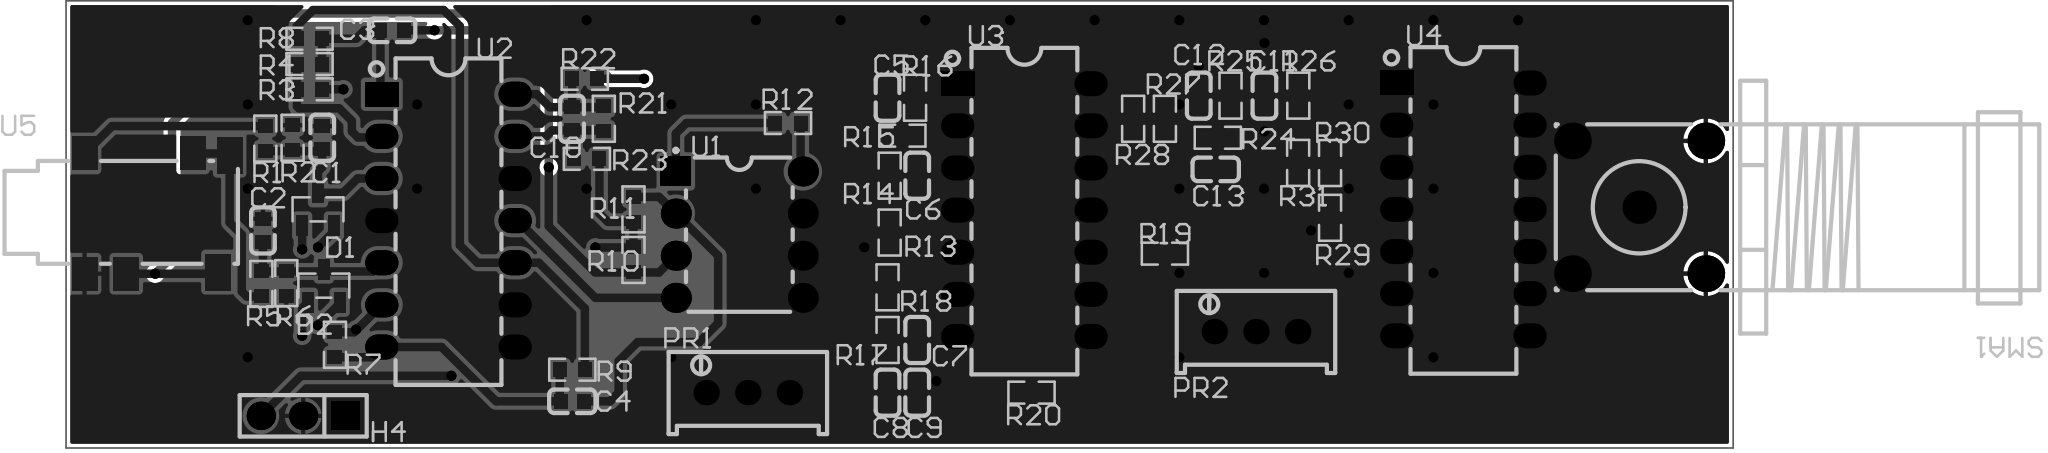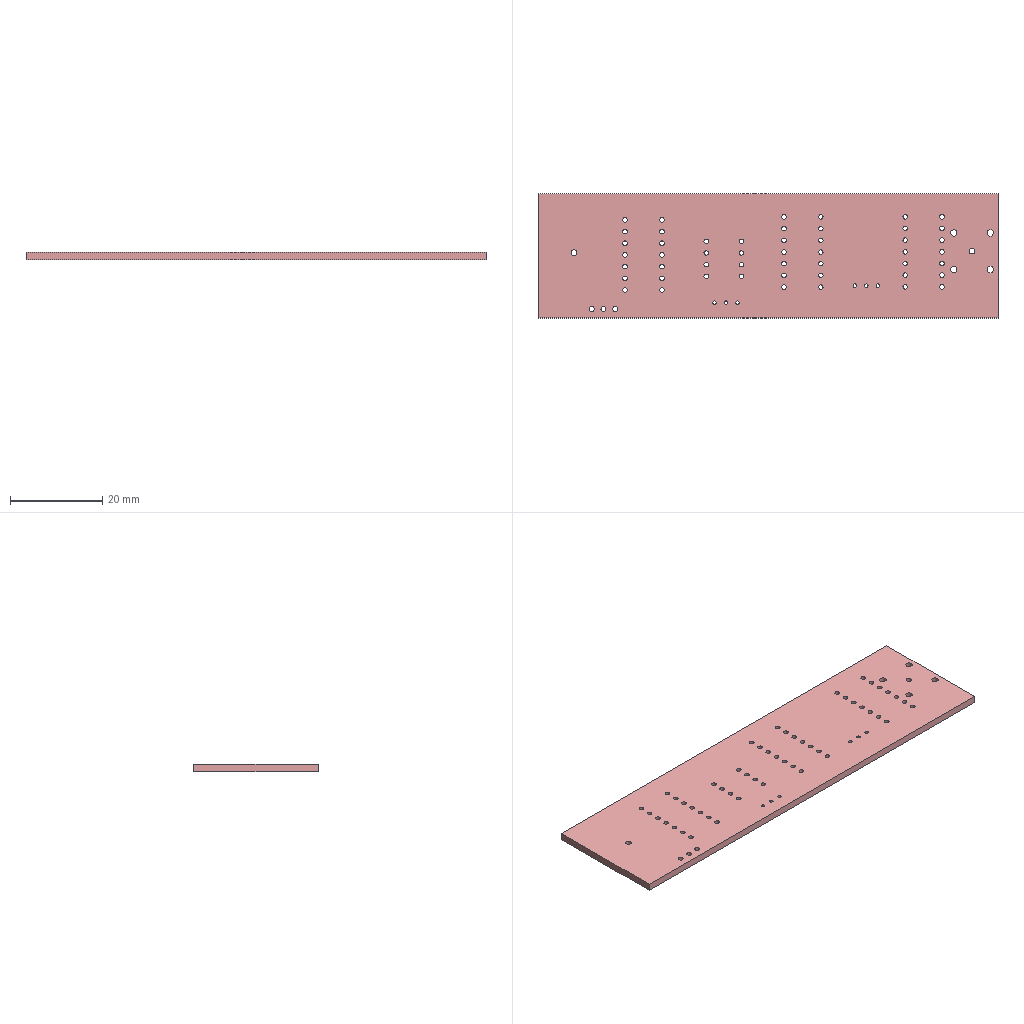Circuit board layout | Altium Designer | box 100 x 27 x 1.6 mm
Layer stack:
# Altium Designer layer stack of  (unit mm; dielectric type: 0 none, 1 core, 2 prepreg, 3 surface material)
index,name,kind,layer,copper_thickness_mm,dielectric_type,dielectric_thickness_mm,dielectric_material,dielectric_constant
0,Top Paste Mask Layer,other,,,,,,
1,Top Silkscreen Layer,other,,,,,,
2,Top Solder Mask Layer,dielectric,,,3,0.01,,3.3
3,Top Layer,copper,Top Layer,0.035,,,,
4,Dielectric1,dielectric,,,3,1.51,FR4,4.5
5,Bottom Layer,copper,Bottom Layer,0.035,,,,
6,Bottom Solder Mask Layer,dielectric,,,3,0.01,,3.3
7,Bottom Silkscreen Layer,other,,,,,,
8,Bottom Paste Mask Layer,other,,,,,,
# drill layer pairs: low layer,high layer
drill_pair,Top Layer,Bottom Layer
Part placement:
Designator,Comment,Layer,Footprint,Center-X(mm),Center-Y(mm),Rotation
C1,1nF,TopLayer,C0603,96.266,106.934,270
C2,1nF,TopLayer,C0603,92.71,101.346,270
C3,330nF,TopLayer,C0603,100.457,113.411,0
C4,330nF,TopLayer,C0603,111.265,91.046,0
C5,470nF,TopLayer,C0603,130.175,109.347,90
C6,470nF,TopLayer,C0603,131.953,104.648,90
C7,220nF,TopLayer,C0603,131.953,94.742,90
C8,100nF,TopLayer,C0603,130.175,91.567,90
C9,100nF,TopLayer,C0603,131.953,91.567,270
D1,BAV99,TopLayer,SOT-23-3_L2.9-W1.3-P1.90-LS2.4-BR,96.012,102.616,270
D2,BAV99,TopLayer,SOT-23-3_L2.9-W1.3-P1.90-LS2.4-BR,96.361,98.018,270
PR1,10kΩ,TopLayer,R_3296,121.793,91.567,0
R1,51K,TopLayer,R0603,92.851,106.883,270
R2,10M,TopLayer,R0603,94.488,106.934,90
R3,20K,TopLayer,R0603,95.504,109.855,180
R4,10K,TopLayer,R0603,95.504,111.379,180
R5,51K,TopLayer,R0603,92.615,98.121,90
R6,10M,TopLayer,R0603,94.107,98.171,270
R7,10K,TopLayer,R0603,97.029,94.455,90
R8,20K,TopLayer,R0603,95.504,112.903,0
R9,20K,TopLayer,R0603,111.265,92.951,0
R10,10MΩ,TopLayer,R0603,114.935,99.568,270
R11,10MΩ,TopLayer,R0603,114.935,102.616,270
R12,5K,TopLayer,R0603,124.206,107.823,0
R13,15K,TopLayer,R0603,130.302,101.219,90
R14,15K,TopLayer,R0603,130.302,104.648,90
R15,10K,TopLayer,R0603,131.064,107.061,0
R16,10K,TopLayer,R0603,131.826,109.347,270
R17,30K,TopLayer,R0603,130.175,94.742,90
R18,30K,TopLayer,R0603,130.175,97.917,90
R19,10K,TopLayer,R0603,146.812,99.949,180
R20,5K,TopLayer,R0603,138.811,91.567,180
U1,AD620ANZ,TopLayer,DIP-8_L9.3-W6.4-P2.54-LS7.6-BL,121.285,101.092,270
U2,LM324NG,TopLayer,PDIP-14_L19.7-W6.6-P2.54-LS8.3-BL,103.839,101.939,270
U3,LM324NG,TopLayer,PDIP-14_L19.7-W6.6-P2.54-LS8.3-BL,138.385,102.574,270
C10,22nF,TopLayer,C0603,111.252,108.077,270
C11,100nF,TopLayer,C0603,152.781,109.474,270
C12,470nF,TopLayer,C0603,148.844,109.474,270
C13,470nF,TopLayer,C0603,149.86,105.029,180
H4,,TopLayer,HDR-TH_3P-P2.54-V-M,95.123,90.17,180
PR2,20kΩ,TopLayer,R_3296,152.273,95.25,0
R21,10M,TopLayer,R0603,113.157,108.077,270
R22,1M,TopLayer,R0603,112.014,110.49,180
R23,10K,TopLayer,R0603,112.141,105.664,0
R24,15K,TopLayer,R0603,149.987,106.934,0
R25,15K,TopLayer,R0603,150.749,109.474,90
R26,1M,TopLayer,R0603,154.813,109.474,90
R27,10K,TopLayer,R0603,146.812,108.077,270
R28,10K,TopLayer,R0603,144.907,108.077,90
R29,2K,TopLayer,R0603,156.718,102.108,270
R30,20K,TopLayer,R0603,156.718,105.41,270
R31,2K,TopLayer,R0603,154.804,105.419,90
U4,LM324NG,TopLayer,PDIP-14_L19.7-W6.6-P2.54-LS8.3-BL,164.719,102.616,270
SMA1,BNC-9.6,TopLayer,SMA-TH_5P_BNC-9.6,175.26,102.743,180
U5,PJ-342 earphone jack,TopLayer,AUDIO-SMD_PJ-342_C9900012319,86.36,102.362,0
Pad and via stacks:
# Altium Designer via and pad stacks of  (unit mm). Each distinct definition once, with the count of objects using it.
# via: kind,start_layer,end_layer,hole_mm,diameter_mm,mode(0 simple;1 top-mid-bottom;2 full stack),diameter_per_layer,count,example_net
# pad: kind,layer,hole_mm,hole_type(0 round;1 square;2 slot),plating,top_size,top_shape(1 round;2 rect;3 octagon;9 rounded rect),mid_size,bottom_size,mode,footprint,size_per_layer,count,example
pad,Top Layer,0,0,plated,0.8x0.9,2,0.8x0.9,0.8x0.9,0,C0603,,26,C1.2
pad,Top Layer,0,0,plated,1.25x0.7,2,1.25x0.7,1.25x0.7,0,SOT-23-3_L2.9-W1.3-P1.90-LS2.4-BR,,6,D1.1
pad,Top Layer,0,0,plated,0.8065x0.864,2,0.8065x0.864,0.8065x0.864,0,R0603,,62,R1.2
pad,Top Layer,0,0,plated,1.5x2,2,1.5x2,1.5x2,0,AUDIO-SMD_PJ-342_C9900012319,,4,U5.3
pad,Top Layer,0,0,plated,1.5x2.2,2,1.5x2.2,1.5x2.2,0,AUDIO-SMD_PJ-342_C9900012319,,2,U5.5
pad,Multi-Layer,0.762,0,plated,1.524x1.524,1,1.524x1.524,1.524x1.524,0,R_3296,,6,PR1.2
pad,Multi-Layer,1,0,plated,1.8x1.8,2,1.8x1.8,1.8x1.8,0,DIP-8_L9.3-W6.4-P2.54-LS7.6-BL,,1,U1.1
pad,Multi-Layer,1,0,plated,1.8x1.8,1,1.8x1.8,1.8x1.8,0,DIP-8_L9.3-W6.4-P2.54-LS7.6-BL,,7,U1.2
pad,Multi-Layer,1,0,plated,2x1.5,2,2x1.5,2x1.5,0,PDIP-14_L19.7-W6.6-P2.54-LS8.3-BL,,3,U2.1
pad,Multi-Layer,1,0,plated,2x1.5,1,2x1.5,2x1.5,0,PDIP-14_L19.7-W6.6-P2.54-LS8.3-BL,,39,U2.2
pad,Multi-Layer,1.1,0,plated,1.7x1.7,2,1.7x1.7,1.7x1.7,0,HDR-TH_3P-P2.54-V-M,,1,H4.1
pad,Multi-Layer,1.1,0,plated,1.7x1.7,1,1.7x1.7,1.7x1.7,0,HDR-TH_3P-P2.54-V-M,,2,H4.2
pad,Multi-Layer,1.4,0,plated,2.2x2.2,1,2.2x2.2,2.2x2.2,0,SMA-TH_5P_BNC-9.6,,4,SMA1.1
pad,Multi-Layer,1.2,0,plated,2x2,1,2x2,2x2,0,SMA-TH_5P_BNC-9.6,,1,SMA1.5
via,Top Layer,Bottom Layer,0.3048,0.61,0,,53,$1N15
Copper pours:
name,layer,net,type(0 solid;1 hatched;2 none)
Top Layer-GND,Top Layer,GND,0
Bottom Layer-GND,Bottom Layer,GND,0